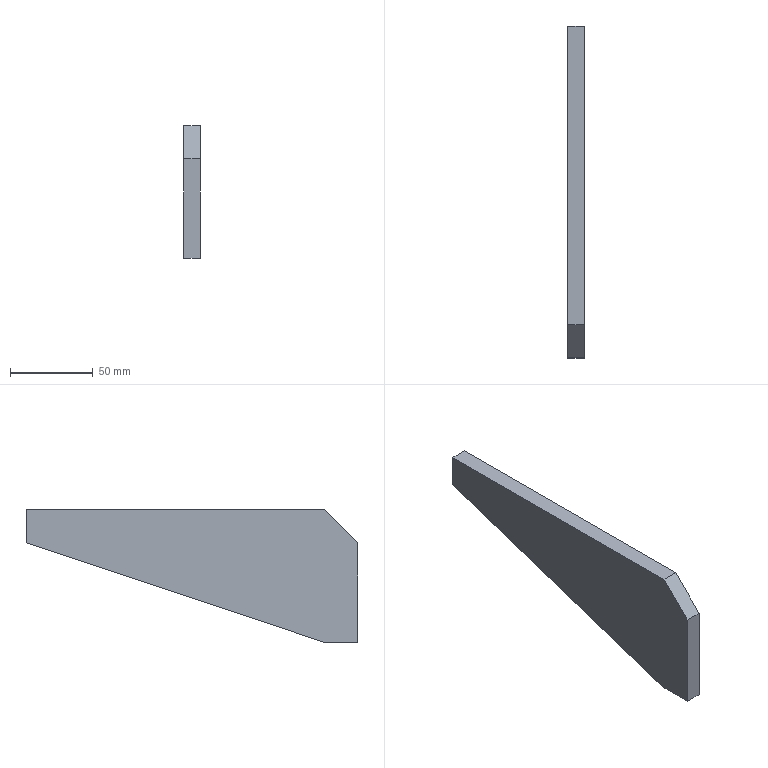Part | SolidWorks | features Extrusion 1 | 1 solid | 8 faces | box 10 x 200 x 80 mm | volume 104000 mm3 | plane 8
STEP:
#1=CARTESIAN_POINT('',(0.,-80.,40.));
#2=VERTEX_POINT('',#1);
#3=CARTESIAN_POINT('',(0.,100.,40.));
#4=VERTEX_POINT('',#3);
#5=CARTESIAN_POINT('',(0.,0.,40.));
#6=DIRECTION('',(0.,1.,0.));
#7=VECTOR('',#6,1000.);
#8=LINE('',#5,#7);
#9=EDGE_CURVE('',#2,#4,#8,.T.);
#10=ORIENTED_EDGE('',*,*,#9,.F.);
#11=CARTESIAN_POINT('',(10.,-80.,40.));
#12=VERTEX_POINT('',#11);
#13=CARTESIAN_POINT('',(10.,-80.,40.));
#14=DIRECTION('',(-1.,0.,0.));
#15=VECTOR('',#14,1000.);
#16=LINE('',#13,#15);
#17=EDGE_CURVE('',#12,#2,#16,.T.);
#18=ORIENTED_EDGE('',*,*,#17,.F.);
#19=CARTESIAN_POINT('',(10.,100.,40.));
#20=VERTEX_POINT('',#19);
#21=CARTESIAN_POINT('',(10.,0.,40.));
#22=DIRECTION('',(0.,1.,0.));
#23=VECTOR('',#22,1000.);
#24=LINE('',#21,#23);
#25=EDGE_CURVE('',#12,#20,#24,.T.);
#26=ORIENTED_EDGE('',*,*,#25,.T.);
#27=CARTESIAN_POINT('',(10.,100.,40.));
#28=DIRECTION('',(-1.,0.,0.));
#29=VECTOR('',#28,1000.);
#30=LINE('',#27,#29);
#31=EDGE_CURVE('',#20,#4,#30,.T.);
#32=ORIENTED_EDGE('',*,*,#31,.T.);
#33=EDGE_LOOP('',(#10,#18,#26,#32));
#34=FACE_OUTER_BOUND('',#33,.T.);
#35=CARTESIAN_POINT('',(10.,0.,40.));
#36=DIRECTION('',(0.,0.,1.));
#37=DIRECTION('',(1.,0.,0.));
#38=AXIS2_PLACEMENT_3D('',#35,#36,#37);
#39=PLANE('',#38);
#40=ADVANCED_FACE('',(#34),#39,.T.);
#41=CARTESIAN_POINT('',(0.,-100.,20.));
#42=VERTEX_POINT('',#41);
#43=CARTESIAN_POINT('',(0.,-60.,60.));
#44=DIRECTION('',(0.,-0.7071,-0.7071));
#45=VECTOR('',#44,1000.);
#46=LINE('',#43,#45);
#47=EDGE_CURVE('',#2,#42,#46,.T.);
#48=ORIENTED_EDGE('',*,*,#47,.T.);
#49=CARTESIAN_POINT('',(10.,-100.,20.));
#50=VERTEX_POINT('',#49);
#51=CARTESIAN_POINT('',(10.,-100.,20.));
#52=DIRECTION('',(-1.,0.,0.));
#53=VECTOR('',#52,1000.);
#54=LINE('',#51,#53);
#55=EDGE_CURVE('',#50,#42,#54,.T.);
#56=ORIENTED_EDGE('',*,*,#55,.F.);
#57=CARTESIAN_POINT('',(10.,-60.,60.));
#58=DIRECTION('',(0.,-0.7071,-0.7071));
#59=VECTOR('',#58,1000.);
#60=LINE('',#57,#59);
#61=EDGE_CURVE('',#12,#50,#60,.T.);
#62=ORIENTED_EDGE('',*,*,#61,.F.);
#63=ORIENTED_EDGE('',*,*,#17,.T.);
#64=EDGE_LOOP('',(#48,#56,#62,#63));
#65=FACE_OUTER_BOUND('',#64,.T.);
#66=CARTESIAN_POINT('',(10.,-60.,60.));
#67=DIRECTION('',(0.,0.7071,-0.7071));
#68=DIRECTION('',(0.,0.7071,0.7071));
#69=AXIS2_PLACEMENT_3D('',#66,#67,#68);
#70=PLANE('',#69);
#71=ADVANCED_FACE('',(#65),#70,.F.);
#72=CARTESIAN_POINT('',(0.,-100.,-40.));
#73=VERTEX_POINT('',#72);
#74=CARTESIAN_POINT('',(0.,-100.,0.));
#75=DIRECTION('',(0.,0.,-1.));
#76=VECTOR('',#75,1000.);
#77=LINE('',#74,#76);
#78=EDGE_CURVE('',#42,#73,#77,.T.);
#79=ORIENTED_EDGE('',*,*,#78,.T.);
#80=CARTESIAN_POINT('',(10.,-100.,-40.));
#81=VERTEX_POINT('',#80);
#82=CARTESIAN_POINT('',(10.,-100.,-40.));
#83=DIRECTION('',(-1.,0.,0.));
#84=VECTOR('',#83,1000.);
#85=LINE('',#82,#84);
#86=EDGE_CURVE('',#81,#73,#85,.T.);
#87=ORIENTED_EDGE('',*,*,#86,.F.);
#88=CARTESIAN_POINT('',(10.,-100.,0.));
#89=DIRECTION('',(0.,0.,-1.));
#90=VECTOR('',#89,1000.);
#91=LINE('',#88,#90);
#92=EDGE_CURVE('',#50,#81,#91,.T.);
#93=ORIENTED_EDGE('',*,*,#92,.F.);
#94=ORIENTED_EDGE('',*,*,#55,.T.);
#95=EDGE_LOOP('',(#79,#87,#93,#94));
#96=FACE_OUTER_BOUND('',#95,.T.);
#97=CARTESIAN_POINT('',(10.,-100.,0.));
#98=DIRECTION('',(0.,1.,0.));
#99=DIRECTION('',(0.,0.,1.));
#100=AXIS2_PLACEMENT_3D('',#97,#98,#99);
#101=PLANE('',#100);
#102=ADVANCED_FACE('',(#96),#101,.F.);
#103=CARTESIAN_POINT('',(0.,-80.,-40.));
#104=VERTEX_POINT('',#103);
#105=CARTESIAN_POINT('',(0.,0.,-40.));
#106=DIRECTION('',(0.,1.,0.));
#107=VECTOR('',#106,1000.);
#108=LINE('',#105,#107);
#109=EDGE_CURVE('',#73,#104,#108,.T.);
#110=ORIENTED_EDGE('',*,*,#109,.T.);
#111=CARTESIAN_POINT('',(10.,-80.,-40.));
#112=VERTEX_POINT('',#111);
#113=CARTESIAN_POINT('',(10.,-80.,-40.));
#114=DIRECTION('',(-1.,0.,0.));
#115=VECTOR('',#114,1000.);
#116=LINE('',#113,#115);
#117=EDGE_CURVE('',#112,#104,#116,.T.);
#118=ORIENTED_EDGE('',*,*,#117,.F.);
#119=CARTESIAN_POINT('',(10.,0.,-40.));
#120=DIRECTION('',(0.,1.,0.));
#121=VECTOR('',#120,1000.);
#122=LINE('',#119,#121);
#123=EDGE_CURVE('',#81,#112,#122,.T.);
#124=ORIENTED_EDGE('',*,*,#123,.F.);
#125=ORIENTED_EDGE('',*,*,#86,.T.);
#126=EDGE_LOOP('',(#110,#118,#124,#125));
#127=FACE_OUTER_BOUND('',#126,.T.);
#128=CARTESIAN_POINT('',(10.,0.,-40.));
#129=DIRECTION('',(0.,0.,1.));
#130=DIRECTION('',(1.,0.,0.));
#131=AXIS2_PLACEMENT_3D('',#128,#129,#130);
#132=PLANE('',#131);
#133=ADVANCED_FACE('',(#127),#132,.F.);
#134=CARTESIAN_POINT('',(0.,100.,20.));
#135=VERTEX_POINT('',#134);
#136=CARTESIAN_POINT('',(0.,4.,-12.));
#137=DIRECTION('',(0.,-0.9487,-0.3162));
#138=VECTOR('',#137,1000.);
#139=LINE('',#136,#138);
#140=EDGE_CURVE('',#135,#104,#139,.T.);
#141=ORIENTED_EDGE('',*,*,#140,.F.);
#142=CARTESIAN_POINT('',(10.,100.,20.));
#143=VERTEX_POINT('',#142);
#144=CARTESIAN_POINT('',(10.,100.,20.));
#145=DIRECTION('',(-1.,0.,0.));
#146=VECTOR('',#145,1000.);
#147=LINE('',#144,#146);
#148=EDGE_CURVE('',#143,#135,#147,.T.);
#149=ORIENTED_EDGE('',*,*,#148,.F.);
#150=CARTESIAN_POINT('',(10.,4.,-12.));
#151=DIRECTION('',(0.,-0.9487,-0.3162));
#152=VECTOR('',#151,1000.);
#153=LINE('',#150,#152);
#154=EDGE_CURVE('',#143,#112,#153,.T.);
#155=ORIENTED_EDGE('',*,*,#154,.T.);
#156=ORIENTED_EDGE('',*,*,#117,.T.);
#157=EDGE_LOOP('',(#141,#149,#155,#156));
#158=FACE_OUTER_BOUND('',#157,.T.);
#159=CARTESIAN_POINT('',(10.,4.,-12.));
#160=DIRECTION('',(0.,0.3162,-0.9487));
#161=DIRECTION('',(0.,0.9487,0.3162));
#162=AXIS2_PLACEMENT_3D('',#159,#160,#161);
#163=PLANE('',#162);
#164=ADVANCED_FACE('',(#158),#163,.T.);
#165=CARTESIAN_POINT('',(0.,100.,0.));
#166=DIRECTION('',(0.,0.,-1.));
#167=VECTOR('',#166,1000.);
#168=LINE('',#165,#167);
#169=EDGE_CURVE('',#4,#135,#168,.T.);
#170=ORIENTED_EDGE('',*,*,#169,.F.);
#171=ORIENTED_EDGE('',*,*,#31,.F.);
#172=CARTESIAN_POINT('',(10.,100.,0.));
#173=DIRECTION('',(0.,0.,-1.));
#174=VECTOR('',#173,1000.);
#175=LINE('',#172,#174);
#176=EDGE_CURVE('',#20,#143,#175,.T.);
#177=ORIENTED_EDGE('',*,*,#176,.T.);
#178=ORIENTED_EDGE('',*,*,#148,.T.);
#179=EDGE_LOOP('',(#170,#171,#177,#178));
#180=FACE_OUTER_BOUND('',#179,.T.);
#181=CARTESIAN_POINT('',(10.,100.,0.));
#182=DIRECTION('',(0.,1.,0.));
#183=DIRECTION('',(0.,0.,1.));
#184=AXIS2_PLACEMENT_3D('',#181,#182,#183);
#185=PLANE('',#184);
#186=ADVANCED_FACE('',(#180),#185,.T.);
#187=ORIENTED_EDGE('',*,*,#25,.F.);
#188=ORIENTED_EDGE('',*,*,#61,.T.);
#189=ORIENTED_EDGE('',*,*,#92,.T.);
#190=ORIENTED_EDGE('',*,*,#123,.T.);
#191=ORIENTED_EDGE('',*,*,#154,.F.);
#192=ORIENTED_EDGE('',*,*,#176,.F.);
#193=EDGE_LOOP('',(#187,#188,#189,#190,#191,#192));
#194=FACE_OUTER_BOUND('',#193,.T.);
#195=CARTESIAN_POINT('',(10.,0.,0.));
#196=DIRECTION('',(1.,0.,0.));
#197=DIRECTION('',(0.,0.,-1.));
#198=AXIS2_PLACEMENT_3D('',#195,#196,#197);
#199=PLANE('',#198);
#200=ADVANCED_FACE('',(#194),#199,.T.);
#201=ORIENTED_EDGE('',*,*,#9,.T.);
#202=ORIENTED_EDGE('',*,*,#169,.T.);
#203=ORIENTED_EDGE('',*,*,#140,.T.);
#204=ORIENTED_EDGE('',*,*,#109,.F.);
#205=ORIENTED_EDGE('',*,*,#78,.F.);
#206=ORIENTED_EDGE('',*,*,#47,.F.);
#207=EDGE_LOOP('',(#201,#202,#203,#204,#205,#206));
#208=FACE_OUTER_BOUND('',#207,.T.);
#209=CARTESIAN_POINT('',(0.,0.,0.));
#210=DIRECTION('',(1.,0.,0.));
#211=DIRECTION('',(0.,0.,-1.));
#212=AXIS2_PLACEMENT_3D('',#209,#210,#211);
#213=PLANE('',#212);
#214=ADVANCED_FACE('',(#208),#213,.F.);
#215=CLOSED_SHELL('',(#40,#71,#102,#133,#164,#186,#200,#214));
#216=MANIFOLD_SOLID_BREP('',#215);
#217=CARTESIAN_POINT('',(0.,0.,0.));
#218=DIRECTION('',(0.,0.,1.));
#219=DIRECTION('',(1.,0.,0.));
#220=AXIS2_PLACEMENT_3D('',#217,#218,#219);
#221=(LENGTH_UNIT()NAMED_UNIT(*)SI_UNIT(.MILLI.,.METRE.));
#222=UNCERTAINTY_MEASURE_WITH_UNIT(LENGTH_MEASURE(0.00001),#221,'','');
#223=(NAMED_UNIT(*)PLANE_ANGLE_UNIT()SI_UNIT($,.RADIAN.));
#224=(NAMED_UNIT(*)SI_UNIT($,.STERADIAN.)SOLID_ANGLE_UNIT());
#225=(GEOMETRIC_REPRESENTATION_CONTEXT(3)GLOBAL_UNCERTAINTY_ASSIGNED_CONTEXT((#222))GLOBAL_UNIT_ASSIGNED_CONTEXT((#221,#223,#224))REPRESENTATION_CONTEXT('',''));
#226=ADVANCED_BREP_SHAPE_REPRESENTATION('',(#216,#220),#225);